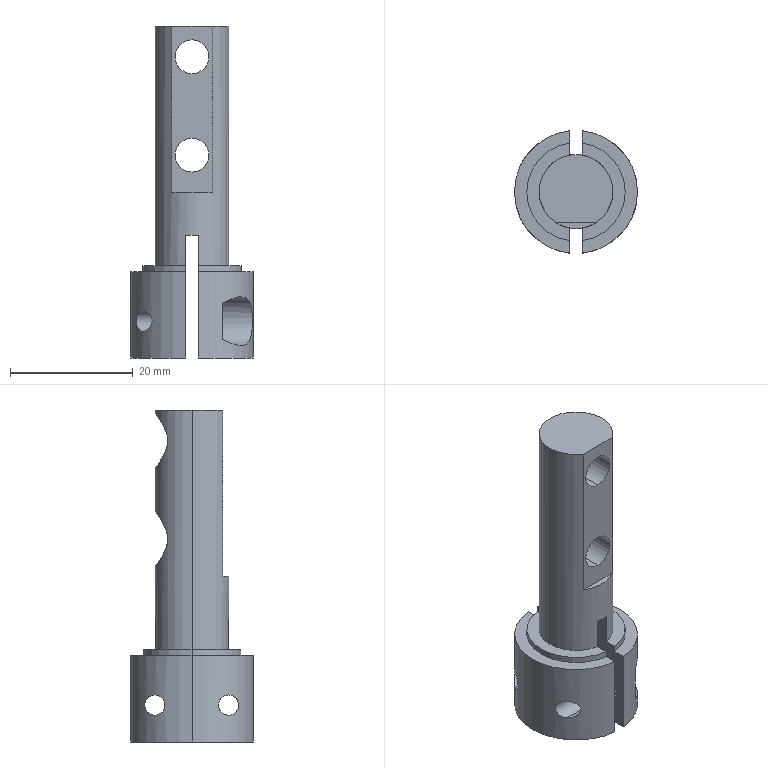Part | SolidWorks | features ICE 8, HoleWzd 3, Extrusion 1 | 1 solid | 51 faces | box 20 x 19.9 x 54 mm | volume 6398 mm3 | cylinder 30 | plane 19 | cone 2 | commonest cylinder face diameters 3.3 x4 4.5 x4 5.5 x4 9 x4 6.35 x3 8 x3